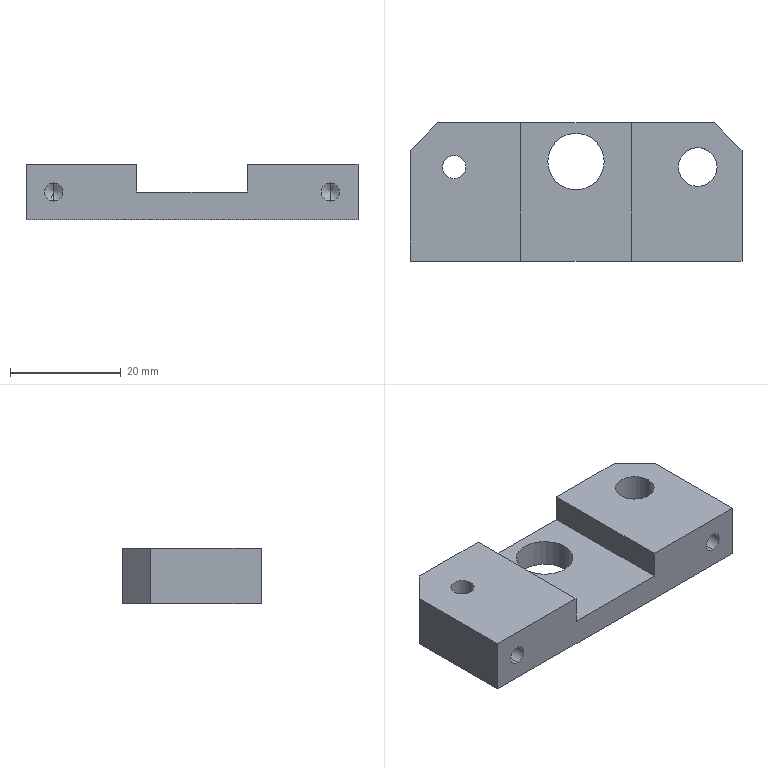Part | STEP file | 2076 Cylinder mounting plate | 1 solid | 26 faces | box 60 x 25 x 10 mm | volume 11081 mm3 | plane 12 | cylinder 10 | cone 4 | commonest cylinder face diameters 3.3 x4 4.2 x2 7 x2 10.2 x2